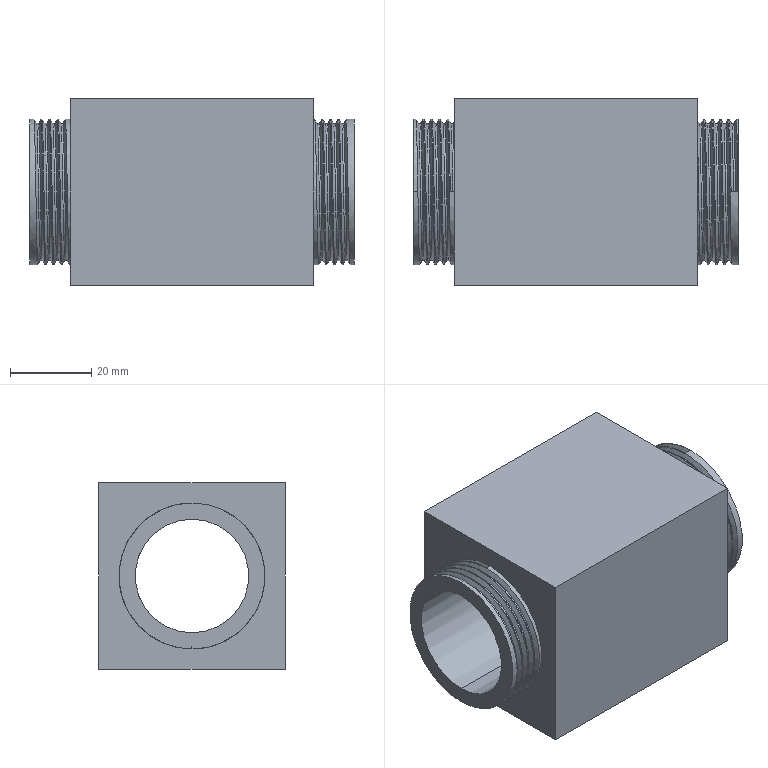Part | SolidWorks | features ICE 2, SweepThread 2, 3DProfileFeature 1, Extrusion 1, HoleWzd 1, RefPoint 1 | 1 solid | 51 faces | box 80 x 46 x 46 mm | volume 94053 mm3 | cylinder 26 | plane 12 | spline 8 | cone 5 | commonest cylinder face diameters 36 x22 19 x2 28 x2